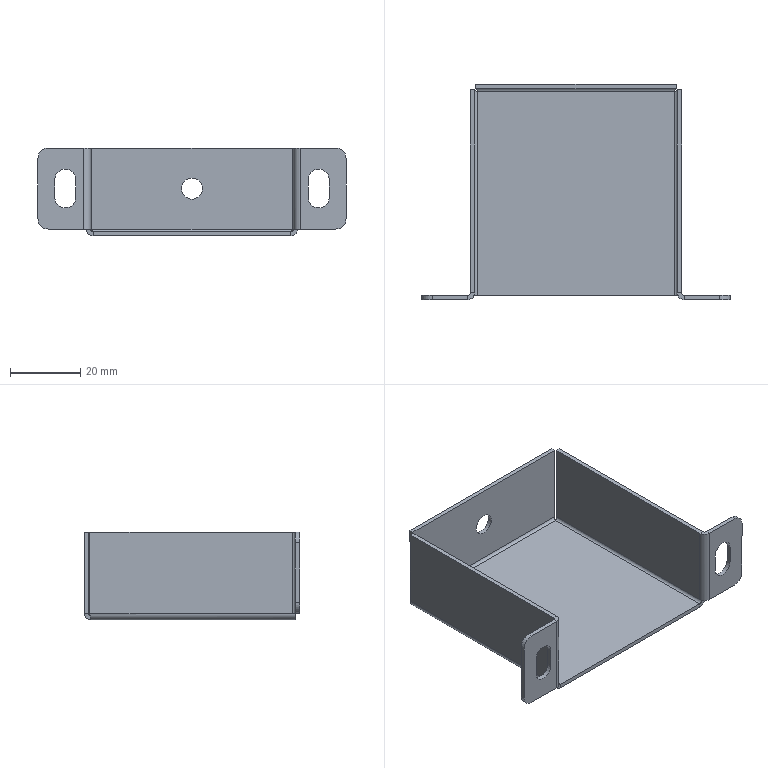Part | SolidWorks | features EdgeFlange 2, Fillet 1, FlatPattern 1, ICE 1, SMBaseFlange 1, SheetMetal 1 | 1 solid | 62 faces | box 87.6 x 61.2 x 25 mm | volume 9770 mm3 | plane 38 | cylinder 20 | spline 4 | commonest cylinder face diameters 6 x10 1.5 x5 3.9 x5